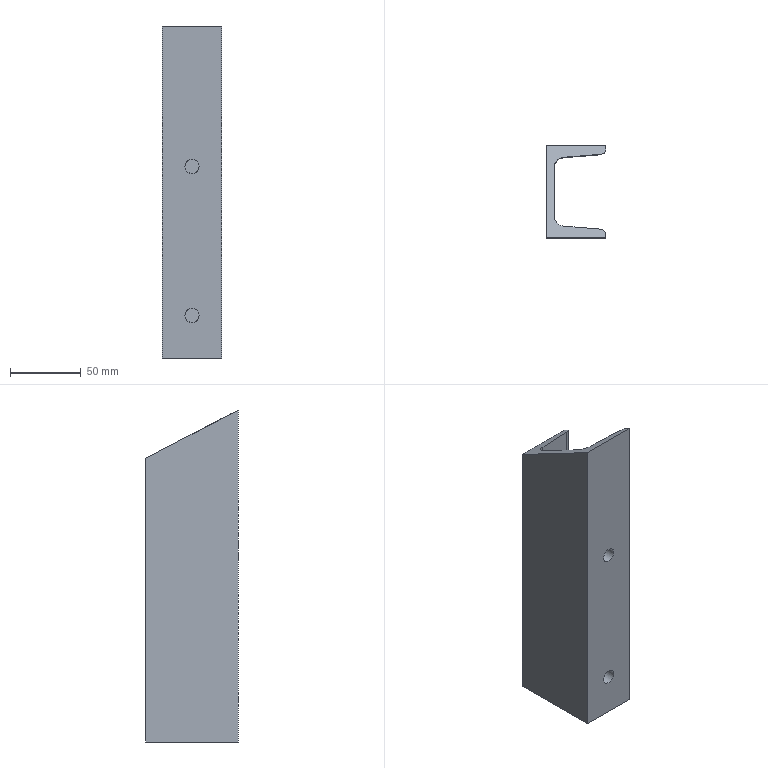Part | STEP file | DIN 1026-1 U 65 1785415623013 | 1 solid | 16 faces | box 42 x 65 x 234.079 mm | volume 194862 mm3 | plane 10 | cylinder 6 | commonest cylinder face diameters 8 x2 10 x2 15 x2
STEP:
#1=CARTESIAN_POINT('',(16.,-32.5,135.));
#2=VERTEX_POINT('',#1);
#3=CARTESIAN_POINT('',(21.,-32.5,135.));
#4=DIRECTION('',(0.,1.,0.));
#5=DIRECTION('',(1.,0.,0.));
#6=AXIS2_PLACEMENT_3D('',#3,#4,#5);
#7=CIRCLE('',#6,5.);
#8=EDGE_CURVE('',#2,#2,#7,.T.);
#9=ORIENTED_EDGE('',*,*,#8,.F.);
#10=CARTESIAN_POINT('',(16.,-24.6,135.));
#11=VERTEX_POINT('',#10);
#12=CARTESIAN_POINT('',(16.,-32.5,135.));
#13=DIRECTION('',(0.,1.,0.));
#14=VECTOR('',#13,5.);
#15=LINE('',#12,#14);
#16=EDGE_CURVE('',#2,#11,#15,.T.);
#17=ORIENTED_EDGE('',*,*,#16,.T.);
#18=CARTESIAN_POINT('',(21.,-25.,135.));
#19=DIRECTION('',(-0.07975,-0.9968,0.));
#20=DIRECTION('',(0.9968,-0.07975,0.));
#21=AXIS2_PLACEMENT_3D('',#18,#19,#20);
#22=ELLIPSE('',#21,5.016,5.);
#23=EDGE_CURVE('',#11,#11,#22,.T.);
#24=ORIENTED_EDGE('',*,*,#23,.F.);
#25=ORIENTED_EDGE('',*,*,#16,.F.);
#26=EDGE_LOOP('',(#9,#17,#24,#25));
#27=FACE_OUTER_BOUND('',#26,.T.);
#28=CARTESIAN_POINT('',(21.,-32.5,135.));
#29=DIRECTION('',(0.,1.,0.));
#30=DIRECTION('',(1.,0.,0.));
#31=AXIS2_PLACEMENT_3D('',#28,#29,#30);
#32=CYLINDRICAL_SURFACE('',#31,5.);
#33=ADVANCED_FACE('',(#27),#32,.F.);
#34=CARTESIAN_POINT('',(16.,-32.5,30.));
#35=VERTEX_POINT('',#34);
#36=CARTESIAN_POINT('',(21.,-32.5,30.));
#37=DIRECTION('',(0.,1.,0.));
#38=DIRECTION('',(1.,0.,0.));
#39=AXIS2_PLACEMENT_3D('',#36,#37,#38);
#40=CIRCLE('',#39,5.);
#41=EDGE_CURVE('',#35,#35,#40,.T.);
#42=ORIENTED_EDGE('',*,*,#41,.F.);
#43=CARTESIAN_POINT('',(16.,-24.6,30.));
#44=VERTEX_POINT('',#43);
#45=CARTESIAN_POINT('',(16.,-32.5,30.));
#46=DIRECTION('',(0.,1.,0.));
#47=VECTOR('',#46,5.);
#48=LINE('',#45,#47);
#49=EDGE_CURVE('',#35,#44,#48,.T.);
#50=ORIENTED_EDGE('',*,*,#49,.T.);
#51=CARTESIAN_POINT('',(21.,-25.,30.));
#52=DIRECTION('',(-0.07975,-0.9968,0.));
#53=DIRECTION('',(0.9968,-0.07975,0.));
#54=AXIS2_PLACEMENT_3D('',#51,#52,#53);
#55=ELLIPSE('',#54,5.016,5.);
#56=EDGE_CURVE('',#44,#44,#55,.T.);
#57=ORIENTED_EDGE('',*,*,#56,.F.);
#58=ORIENTED_EDGE('',*,*,#49,.F.);
#59=EDGE_LOOP('',(#42,#50,#57,#58));
#60=FACE_OUTER_BOUND('',#59,.T.);
#61=CARTESIAN_POINT('',(21.,-32.5,30.));
#62=DIRECTION('',(0.,1.,0.));
#63=DIRECTION('',(1.,0.,0.));
#64=AXIS2_PLACEMENT_3D('',#61,#62,#63);
#65=CYLINDRICAL_SURFACE('',#64,5.);
#66=ADVANCED_FACE('',(#60),#65,.F.);
#67=CARTESIAN_POINT('',(5.5,-16.836,225.866));
#68=VERTEX_POINT('',#67);
#69=CARTESIAN_POINT('',(12.402,-24.312,229.786));
#70=VERTEX_POINT('',#69);
#71=CARTESIAN_POINT('',(13.,-16.836,225.866));
#72=DIRECTION('',(0.,0.4643,0.8857));
#73=DIRECTION('',(0.,-0.8857,0.4643));
#74=AXIS2_PLACEMENT_3D('',#71,#72,#73);
#75=ELLIPSE('',#74,8.468,7.5);
#76=EDGE_CURVE('',#68,#70,#75,.T.);
#77=ORIENTED_EDGE('',*,*,#76,.F.);
#78=CARTESIAN_POINT('',(5.5,16.836,208.212));
#79=VERTEX_POINT('',#78);
#80=CARTESIAN_POINT('',(5.5,89.257,170.243));
#81=DIRECTION('',(0.,-0.8857,0.4643));
#82=VECTOR('',#81,10.);
#83=LINE('',#80,#82);
#84=EDGE_CURVE('',#79,#68,#83,.T.);
#85=ORIENTED_EDGE('',*,*,#84,.F.);
#86=CARTESIAN_POINT('',(12.402,24.312,204.293));
#87=VERTEX_POINT('',#86);
#88=CARTESIAN_POINT('',(13.,16.836,208.212));
#89=DIRECTION('',(0.,0.4643,0.8857));
#90=DIRECTION('',(0.,0.8857,-0.4643));
#91=AXIS2_PLACEMENT_3D('',#88,#89,#90);
#92=ELLIPSE('',#91,8.468,7.5);
#93=EDGE_CURVE('',#87,#79,#92,.T.);
#94=ORIENTED_EDGE('',*,*,#93,.F.);
#95=CARTESIAN_POINT('',(38.319,26.386,203.206));
#96=VERTEX_POINT('',#95);
#97=CARTESIAN_POINT('',(26.722,25.458,203.692));
#98=DIRECTION('',(-0.9959,-0.07968,0.04177));
#99=VECTOR('',#98,10.);
#100=LINE('',#97,#99);
#101=EDGE_CURVE('',#96,#87,#100,.T.);
#102=ORIENTED_EDGE('',*,*,#101,.F.);
#103=CARTESIAN_POINT('',(42.,30.373,201.115));
#104=VERTEX_POINT('',#103);
#105=CARTESIAN_POINT('',(38.,30.373,201.115));
#106=DIRECTION('',(0.,-0.4643,-0.8857));
#107=DIRECTION('',(0.,0.8857,-0.4643));
#108=AXIS2_PLACEMENT_3D('',#105,#106,#107);
#109=ELLIPSE('',#108,4.516,4.);
#110=EDGE_CURVE('',#104,#96,#109,.T.);
#111=ORIENTED_EDGE('',*,*,#110,.F.);
#112=CARTESIAN_POINT('',(42.,32.5,200.));
#113=VERTEX_POINT('',#112);
#114=CARTESIAN_POINT('',(42.,102.003,163.56));
#115=DIRECTION('',(0.,-0.8857,0.4643));
#116=VECTOR('',#115,10.);
#117=LINE('',#114,#116);
#118=EDGE_CURVE('',#113,#104,#117,.T.);
#119=ORIENTED_EDGE('',*,*,#118,.F.);
#120=CARTESIAN_POINT('',(0.,32.5,200.));
#121=VERTEX_POINT('',#120);
#122=CARTESIAN_POINT('',(0.,32.5,200.));
#123=DIRECTION('',(1.,0.,0.));
#124=VECTOR('',#123,10.);
#125=LINE('',#122,#124);
#126=EDGE_CURVE('',#121,#113,#125,.T.);
#127=ORIENTED_EDGE('',*,*,#126,.F.);
#128=CARTESIAN_POINT('',(0.,-32.5,234.079));
#129=VERTEX_POINT('',#128);
#130=CARTESIAN_POINT('',(0.,89.257,170.243));
#131=DIRECTION('',(0.,0.8857,-0.4643));
#132=VECTOR('',#131,10.);
#133=LINE('',#130,#132);
#134=EDGE_CURVE('',#129,#121,#133,.T.);
#135=ORIENTED_EDGE('',*,*,#134,.F.);
#136=CARTESIAN_POINT('',(42.,-32.5,234.079));
#137=VERTEX_POINT('',#136);
#138=CARTESIAN_POINT('',(31.5,-32.5,234.079));
#139=DIRECTION('',(-1.,0.,0.));
#140=VECTOR('',#139,10.);
#141=LINE('',#138,#140);
#142=EDGE_CURVE('',#137,#129,#141,.T.);
#143=ORIENTED_EDGE('',*,*,#142,.F.);
#144=CARTESIAN_POINT('',(42.,-30.373,232.963));
#145=VERTEX_POINT('',#144);
#146=CARTESIAN_POINT('',(42.,77.345,176.488));
#147=DIRECTION('',(0.,-0.8857,0.4643));
#148=VECTOR('',#147,10.);
#149=LINE('',#146,#148);
#150=EDGE_CURVE('',#145,#137,#149,.T.);
#151=ORIENTED_EDGE('',*,*,#150,.F.);
#152=CARTESIAN_POINT('',(38.319,-26.386,230.873));
#153=VERTEX_POINT('',#152);
#154=CARTESIAN_POINT('',(38.,-30.373,232.963));
#155=DIRECTION('',(0.,-0.4643,-0.8857));
#156=DIRECTION('',(0.,-0.8857,0.4643));
#157=AXIS2_PLACEMENT_3D('',#154,#155,#156);
#158=ELLIPSE('',#157,4.516,4.);
#159=EDGE_CURVE('',#153,#145,#158,.T.);
#160=ORIENTED_EDGE('',*,*,#159,.F.);
#161=CARTESIAN_POINT('',(-4.273,-22.978,229.087));
#162=DIRECTION('',(0.9959,-0.07968,0.04177));
#163=VECTOR('',#162,10.);
#164=LINE('',#161,#163);
#165=EDGE_CURVE('',#70,#153,#164,.T.);
#166=ORIENTED_EDGE('',*,*,#165,.F.);
#167=EDGE_LOOP('',(#77,#85,#94,#102,#111,#119,#127,#135,#143,#151,#160,#166));
#168=FACE_OUTER_BOUND('',#167,.T.);
#169=CARTESIAN_POINT('',(0.,89.257,170.243));
#170=DIRECTION('',(0.,-0.4643,-0.8857));
#171=DIRECTION('',(-1.,0.,0.));
#172=AXIS2_PLACEMENT_3D('',#169,#170,#171);
#173=PLANE('',#172);
#174=ADVANCED_FACE('',(#168),#173,.F.);
#175=ORIENTED_EDGE('',*,*,#126,.T.);
#176=CARTESIAN_POINT('',(42.,32.5,0.));
#177=VERTEX_POINT('',#176);
#178=CARTESIAN_POINT('',(42.,32.5,0.));
#179=DIRECTION('',(0.,0.,1.));
#180=VECTOR('',#179,10.);
#181=LINE('',#178,#180);
#182=EDGE_CURVE('',#177,#113,#181,.T.);
#183=ORIENTED_EDGE('',*,*,#182,.F.);
#184=CARTESIAN_POINT('',(0.,32.5,0.));
#185=VERTEX_POINT('',#184);
#186=CARTESIAN_POINT('',(10.5,32.5,0.));
#187=DIRECTION('',(1.,0.,0.));
#188=VECTOR('',#187,10.);
#189=LINE('',#186,#188);
#190=EDGE_CURVE('',#185,#177,#189,.T.);
#191=ORIENTED_EDGE('',*,*,#190,.F.);
#192=CARTESIAN_POINT('',(0.,32.5,0.));
#193=DIRECTION('',(0.,0.,1.));
#194=VECTOR('',#193,10.);
#195=LINE('',#192,#194);
#196=EDGE_CURVE('',#185,#121,#195,.T.);
#197=ORIENTED_EDGE('',*,*,#196,.T.);
#198=EDGE_LOOP('',(#175,#183,#191,#197));
#199=FACE_OUTER_BOUND('',#198,.T.);
#200=CARTESIAN_POINT('',(0.,32.5,0.));
#201=DIRECTION('',(0.,1.,0.));
#202=DIRECTION('',(0.,0.,1.));
#203=AXIS2_PLACEMENT_3D('',#200,#201,#202);
#204=PLANE('',#203);
#205=ADVANCED_FACE('',(#199),#204,.T.);
#206=ORIENTED_EDGE('',*,*,#118,.T.);
#207=CARTESIAN_POINT('',(42.,30.373,0.));
#208=VERTEX_POINT('',#207);
#209=CARTESIAN_POINT('',(42.,30.373,0.));
#210=DIRECTION('',(0.,0.,1.));
#211=VECTOR('',#210,10.);
#212=LINE('',#209,#211);
#213=EDGE_CURVE('',#208,#104,#212,.T.);
#214=ORIENTED_EDGE('',*,*,#213,.F.);
#215=CARTESIAN_POINT('',(42.,16.25,0.));
#216=DIRECTION('',(0.,-1.,0.));
#217=VECTOR('',#216,10.);
#218=LINE('',#215,#217);
#219=EDGE_CURVE('',#177,#208,#218,.T.);
#220=ORIENTED_EDGE('',*,*,#219,.F.);
#221=ORIENTED_EDGE('',*,*,#182,.T.);
#222=EDGE_LOOP('',(#206,#214,#220,#221));
#223=FACE_OUTER_BOUND('',#222,.T.);
#224=CARTESIAN_POINT('',(42.,32.5,0.));
#225=DIRECTION('',(1.,0.,0.));
#226=DIRECTION('',(0.,0.,-1.));
#227=AXIS2_PLACEMENT_3D('',#224,#225,#226);
#228=PLANE('',#227);
#229=ADVANCED_FACE('',(#223),#228,.T.);
#230=ORIENTED_EDGE('',*,*,#110,.T.);
#231=CARTESIAN_POINT('',(38.319,26.386,0.));
#232=VERTEX_POINT('',#231);
#233=CARTESIAN_POINT('',(38.319,26.386,0.));
#234=DIRECTION('',(0.,0.,1.));
#235=VECTOR('',#234,10.);
#236=LINE('',#233,#235);
#237=EDGE_CURVE('',#232,#96,#236,.T.);
#238=ORIENTED_EDGE('',*,*,#237,.F.);
#239=CARTESIAN_POINT('',(38.,30.373,0.));
#240=DIRECTION('',(0.,0.,-1.));
#241=DIRECTION('',(-0.07975,0.9968,0.));
#242=AXIS2_PLACEMENT_3D('',#239,#240,#241);
#243=CIRCLE('',#242,4.);
#244=EDGE_CURVE('',#208,#232,#243,.T.);
#245=ORIENTED_EDGE('',*,*,#244,.F.);
#246=ORIENTED_EDGE('',*,*,#213,.T.);
#247=EDGE_LOOP('',(#230,#238,#245,#246));
#248=FACE_OUTER_BOUND('',#247,.T.);
#249=CARTESIAN_POINT('',(38.,30.373,0.));
#250=DIRECTION('',(0.,0.,1.));
#251=DIRECTION('',(-0.07975,0.9968,0.));
#252=AXIS2_PLACEMENT_3D('',#249,#250,#251);
#253=CYLINDRICAL_SURFACE('',#252,4.);
#254=ADVANCED_FACE('',(#248),#253,.T.);
#255=ORIENTED_EDGE('',*,*,#101,.T.);
#256=CARTESIAN_POINT('',(12.402,24.312,0.));
#257=VERTEX_POINT('',#256);
#258=CARTESIAN_POINT('',(12.402,24.312,0.));
#259=DIRECTION('',(0.,0.,1.));
#260=VECTOR('',#259,10.);
#261=LINE('',#258,#260);
#262=EDGE_CURVE('',#257,#87,#261,.T.);
#263=ORIENTED_EDGE('',*,*,#262,.F.);
#264=CARTESIAN_POINT('',(28.666,25.613,0.));
#265=DIRECTION('',(-0.9968,-0.07975,0.));
#266=VECTOR('',#265,10.);
#267=LINE('',#264,#266);
#268=EDGE_CURVE('',#232,#257,#267,.T.);
#269=ORIENTED_EDGE('',*,*,#268,.F.);
#270=ORIENTED_EDGE('',*,*,#237,.T.);
#271=EDGE_LOOP('',(#255,#263,#269,#270));
#272=FACE_OUTER_BOUND('',#271,.T.);
#273=CARTESIAN_POINT('',(38.319,26.386,0.));
#274=DIRECTION('',(0.07975,-0.9968,0.));
#275=DIRECTION('',(0.,0.,-1.));
#276=AXIS2_PLACEMENT_3D('',#273,#274,#275);
#277=PLANE('',#276);
#278=ADVANCED_FACE('',(#272),#277,.T.);
#279=ORIENTED_EDGE('',*,*,#93,.T.);
#280=CARTESIAN_POINT('',(5.5,16.836,0.));
#281=VERTEX_POINT('',#280);
#282=CARTESIAN_POINT('',(5.5,16.836,0.));
#283=DIRECTION('',(0.,0.,1.));
#284=VECTOR('',#283,10.);
#285=LINE('',#282,#284);
#286=EDGE_CURVE('',#281,#79,#285,.T.);
#287=ORIENTED_EDGE('',*,*,#286,.F.);
#288=CARTESIAN_POINT('',(13.,16.836,0.));
#289=DIRECTION('',(0.,0.,1.));
#290=DIRECTION('',(-0.07975,0.9968,0.));
#291=AXIS2_PLACEMENT_3D('',#288,#289,#290);
#292=CIRCLE('',#291,7.5);
#293=EDGE_CURVE('',#257,#281,#292,.T.);
#294=ORIENTED_EDGE('',*,*,#293,.F.);
#295=ORIENTED_EDGE('',*,*,#262,.T.);
#296=EDGE_LOOP('',(#279,#287,#294,#295));
#297=FACE_OUTER_BOUND('',#296,.T.);
#298=CARTESIAN_POINT('',(13.,16.836,0.));
#299=DIRECTION('',(0.,0.,1.));
#300=DIRECTION('',(-0.07975,0.9968,0.));
#301=AXIS2_PLACEMENT_3D('',#298,#299,#300);
#302=CYLINDRICAL_SURFACE('',#301,7.5);
#303=ADVANCED_FACE('',(#297),#302,.F.);
#304=ORIENTED_EDGE('',*,*,#84,.T.);
#305=CARTESIAN_POINT('',(5.5,-16.836,0.));
#306=VERTEX_POINT('',#305);
#307=CARTESIAN_POINT('',(5.5,-16.836,0.));
#308=DIRECTION('',(0.,0.,1.));
#309=VECTOR('',#308,10.);
#310=LINE('',#307,#309);
#311=EDGE_CURVE('',#306,#68,#310,.T.);
#312=ORIENTED_EDGE('',*,*,#311,.F.);
#313=CARTESIAN_POINT('',(5.5,0.,0.));
#314=DIRECTION('',(0.,-1.,0.));
#315=VECTOR('',#314,10.);
#316=LINE('',#313,#315);
#317=EDGE_CURVE('',#281,#306,#316,.T.);
#318=ORIENTED_EDGE('',*,*,#317,.F.);
#319=ORIENTED_EDGE('',*,*,#286,.T.);
#320=EDGE_LOOP('',(#304,#312,#318,#319));
#321=FACE_OUTER_BOUND('',#320,.T.);
#322=CARTESIAN_POINT('',(5.5,0.,0.));
#323=DIRECTION('',(1.,0.,0.));
#324=DIRECTION('',(0.,0.,-1.));
#325=AXIS2_PLACEMENT_3D('',#322,#323,#324);
#326=PLANE('',#325);
#327=ADVANCED_FACE('',(#321),#326,.T.);
#328=ORIENTED_EDGE('',*,*,#76,.T.);
#329=CARTESIAN_POINT('',(12.402,-24.312,0.));
#330=VERTEX_POINT('',#329);
#331=CARTESIAN_POINT('',(12.402,-24.312,0.));
#332=DIRECTION('',(0.,0.,1.));
#333=VECTOR('',#332,10.);
#334=LINE('',#331,#333);
#335=EDGE_CURVE('',#330,#70,#334,.T.);
#336=ORIENTED_EDGE('',*,*,#335,.F.);
#337=CARTESIAN_POINT('',(13.,-16.836,0.));
#338=DIRECTION('',(0.,0.,1.));
#339=DIRECTION('',(-1.,0.,0.));
#340=AXIS2_PLACEMENT_3D('',#337,#338,#339);
#341=CIRCLE('',#340,7.5);
#342=EDGE_CURVE('',#306,#330,#341,.T.);
#343=ORIENTED_EDGE('',*,*,#342,.F.);
#344=ORIENTED_EDGE('',*,*,#311,.T.);
#345=EDGE_LOOP('',(#328,#336,#343,#344));
#346=FACE_OUTER_BOUND('',#345,.T.);
#347=CARTESIAN_POINT('',(13.,-16.836,0.));
#348=DIRECTION('',(0.,0.,1.));
#349=DIRECTION('',(-1.,0.,0.));
#350=AXIS2_PLACEMENT_3D('',#347,#348,#349);
#351=CYLINDRICAL_SURFACE('',#350,7.5);
#352=ADVANCED_FACE('',(#346),#351,.F.);
#353=ORIENTED_EDGE('',*,*,#165,.T.);
#354=CARTESIAN_POINT('',(38.319,-26.386,0.));
#355=VERTEX_POINT('',#354);
#356=CARTESIAN_POINT('',(38.319,-26.386,0.));
#357=DIRECTION('',(0.,0.,1.));
#358=VECTOR('',#357,10.);
#359=LINE('',#356,#358);
#360=EDGE_CURVE('',#355,#153,#359,.T.);
#361=ORIENTED_EDGE('',*,*,#360,.F.);
#362=CARTESIAN_POINT('',(15.707,-24.577,0.));
#363=DIRECTION('',(0.9968,-0.07975,0.));
#364=VECTOR('',#363,10.);
#365=LINE('',#362,#364);
#366=EDGE_CURVE('',#330,#355,#365,.T.);
#367=ORIENTED_EDGE('',*,*,#366,.F.);
#368=ORIENTED_EDGE('',*,*,#335,.T.);
#369=EDGE_LOOP('',(#353,#361,#367,#368));
#370=FACE_OUTER_BOUND('',#369,.T.);
#371=ORIENTED_EDGE('',*,*,#23,.T.);
#372=EDGE_LOOP('',(#371));
#373=FACE_BOUND('',#372,.T.);
#374=ORIENTED_EDGE('',*,*,#56,.T.);
#375=EDGE_LOOP('',(#374));
#376=FACE_BOUND('',#375,.T.);
#377=CARTESIAN_POINT('',(12.402,-24.312,0.));
#378=DIRECTION('',(0.07975,0.9968,0.));
#379=DIRECTION('',(0.,0.,1.));
#380=AXIS2_PLACEMENT_3D('',#377,#378,#379);
#381=PLANE('',#380);
#382=ADVANCED_FACE('',(#370,#373,#376),#381,.T.);
#383=ORIENTED_EDGE('',*,*,#159,.T.);
#384=CARTESIAN_POINT('',(42.,-30.373,0.));
#385=VERTEX_POINT('',#384);
#386=CARTESIAN_POINT('',(42.,-30.373,0.));
#387=DIRECTION('',(0.,0.,1.));
#388=VECTOR('',#387,10.);
#389=LINE('',#386,#388);
#390=EDGE_CURVE('',#385,#145,#389,.T.);
#391=ORIENTED_EDGE('',*,*,#390,.F.);
#392=CARTESIAN_POINT('',(38.,-30.373,0.));
#393=DIRECTION('',(0.,0.,-1.));
#394=DIRECTION('',(-1.,0.,0.));
#395=AXIS2_PLACEMENT_3D('',#392,#393,#394);
#396=CIRCLE('',#395,4.);
#397=EDGE_CURVE('',#355,#385,#396,.T.);
#398=ORIENTED_EDGE('',*,*,#397,.F.);
#399=ORIENTED_EDGE('',*,*,#360,.T.);
#400=EDGE_LOOP('',(#383,#391,#398,#399));
#401=FACE_OUTER_BOUND('',#400,.T.);
#402=CARTESIAN_POINT('',(38.,-30.373,0.));
#403=DIRECTION('',(0.,0.,1.));
#404=DIRECTION('',(-1.,0.,0.));
#405=AXIS2_PLACEMENT_3D('',#402,#403,#404);
#406=CYLINDRICAL_SURFACE('',#405,4.);
#407=ADVANCED_FACE('',(#401),#406,.T.);
#408=ORIENTED_EDGE('',*,*,#150,.T.);
#409=CARTESIAN_POINT('',(42.,-32.5,0.));
#410=VERTEX_POINT('',#409);
#411=CARTESIAN_POINT('',(42.,-32.5,0.));
#412=DIRECTION('',(0.,0.,1.));
#413=VECTOR('',#412,10.);
#414=LINE('',#411,#413);
#415=EDGE_CURVE('',#410,#137,#414,.T.);
#416=ORIENTED_EDGE('',*,*,#415,.F.);
#417=CARTESIAN_POINT('',(42.,-15.186,0.));
#418=DIRECTION('',(0.,-1.,0.));
#419=VECTOR('',#418,10.);
#420=LINE('',#417,#419);
#421=EDGE_CURVE('',#385,#410,#420,.T.);
#422=ORIENTED_EDGE('',*,*,#421,.F.);
#423=ORIENTED_EDGE('',*,*,#390,.T.);
#424=EDGE_LOOP('',(#408,#416,#422,#423));
#425=FACE_OUTER_BOUND('',#424,.T.);
#426=CARTESIAN_POINT('',(42.,-30.373,0.));
#427=DIRECTION('',(1.,0.,0.));
#428=DIRECTION('',(0.,0.,-1.));
#429=AXIS2_PLACEMENT_3D('',#426,#427,#428);
#430=PLANE('',#429);
#431=ADVANCED_FACE('',(#425),#430,.T.);
#432=ORIENTED_EDGE('',*,*,#142,.T.);
#433=CARTESIAN_POINT('',(0.,-32.5,0.));
#434=VERTEX_POINT('',#433);
#435=CARTESIAN_POINT('',(0.,-32.5,0.));
#436=DIRECTION('',(0.,0.,1.));
#437=VECTOR('',#436,10.);
#438=LINE('',#435,#437);
#439=EDGE_CURVE('',#434,#129,#438,.T.);
#440=ORIENTED_EDGE('',*,*,#439,.F.);
#441=CARTESIAN_POINT('',(31.5,-32.5,0.));
#442=DIRECTION('',(-1.,0.,0.));
#443=VECTOR('',#442,10.);
#444=LINE('',#441,#443);
#445=EDGE_CURVE('',#410,#434,#444,.T.);
#446=ORIENTED_EDGE('',*,*,#445,.F.);
#447=ORIENTED_EDGE('',*,*,#415,.T.);
#448=EDGE_LOOP('',(#432,#440,#446,#447));
#449=FACE_OUTER_BOUND('',#448,.T.);
#450=ORIENTED_EDGE('',*,*,#8,.T.);
#451=EDGE_LOOP('',(#450));
#452=FACE_BOUND('',#451,.T.);
#453=ORIENTED_EDGE('',*,*,#41,.T.);
#454=EDGE_LOOP('',(#453));
#455=FACE_BOUND('',#454,.T.);
#456=CARTESIAN_POINT('',(42.,-32.5,0.));
#457=DIRECTION('',(0.,-1.,0.));
#458=DIRECTION('',(0.,0.,-1.));
#459=AXIS2_PLACEMENT_3D('',#456,#457,#458);
#460=PLANE('',#459);
#461=ADVANCED_FACE('',(#449,#452,#455),#460,.T.);
#462=ORIENTED_EDGE('',*,*,#134,.T.);
#463=ORIENTED_EDGE('',*,*,#196,.F.);
#464=CARTESIAN_POINT('',(0.,0.,0.));
#465=DIRECTION('',(0.,1.,0.));
#466=VECTOR('',#465,10.);
#467=LINE('',#464,#466);
#468=EDGE_CURVE('',#434,#185,#467,.T.);
#469=ORIENTED_EDGE('',*,*,#468,.F.);
#470=ORIENTED_EDGE('',*,*,#439,.T.);
#471=EDGE_LOOP('',(#462,#463,#469,#470));
#472=FACE_OUTER_BOUND('',#471,.T.);
#473=CARTESIAN_POINT('',(0.,0.,0.));
#474=DIRECTION('',(-1.,0.,0.));
#475=DIRECTION('',(0.,0.,1.));
#476=AXIS2_PLACEMENT_3D('',#473,#474,#475);
#477=PLANE('',#476);
#478=ADVANCED_FACE('',(#472),#477,.T.);
#479=ORIENTED_EDGE('',*,*,#190,.T.);
#480=ORIENTED_EDGE('',*,*,#219,.T.);
#481=ORIENTED_EDGE('',*,*,#244,.T.);
#482=ORIENTED_EDGE('',*,*,#268,.T.);
#483=ORIENTED_EDGE('',*,*,#293,.T.);
#484=ORIENTED_EDGE('',*,*,#317,.T.);
#485=ORIENTED_EDGE('',*,*,#342,.T.);
#486=ORIENTED_EDGE('',*,*,#366,.T.);
#487=ORIENTED_EDGE('',*,*,#397,.T.);
#488=ORIENTED_EDGE('',*,*,#421,.T.);
#489=ORIENTED_EDGE('',*,*,#445,.T.);
#490=ORIENTED_EDGE('',*,*,#468,.T.);
#491=EDGE_LOOP('',(#479,#480,#481,#482,#483,#484,#485,#486,#487,#488,#489,#490));
#492=FACE_OUTER_BOUND('',#491,.T.);
#493=CARTESIAN_POINT('',(21.,0.,0.));
#494=DIRECTION('',(0.,0.,1.));
#495=DIRECTION('',(1.,0.,0.));
#496=AXIS2_PLACEMENT_3D('',#493,#494,#495);
#497=PLANE('',#496);
#498=ADVANCED_FACE('',(#492),#497,.F.);
#499=CLOSED_SHELL('',(#33,#66,#174,#205,#229,#254,#278,#303,#327,#352,#382,#407,#431,#461,#478,#498));
#500=MANIFOLD_SOLID_BREP('',#499);
#501=(LENGTH_UNIT()NAMED_UNIT(*)SI_UNIT(.MILLI.,.METRE.));
#502=UNCERTAINTY_MEASURE_WITH_UNIT(LENGTH_MEASURE(0.01),#501,'','');
#503=(NAMED_UNIT(*)PLANE_ANGLE_UNIT()SI_UNIT($,.RADIAN.));
#504=(NAMED_UNIT(*)SI_UNIT($,.STERADIAN.)SOLID_ANGLE_UNIT());
#505=(GEOMETRIC_REPRESENTATION_CONTEXT(3)GLOBAL_UNCERTAINTY_ASSIGNED_CONTEXT((#502))GLOBAL_UNIT_ASSIGNED_CONTEXT((#501,#503,#504))REPRESENTATION_CONTEXT('',''));
#506=ADVANCED_BREP_SHAPE_REPRESENTATION('',(#500),#505);